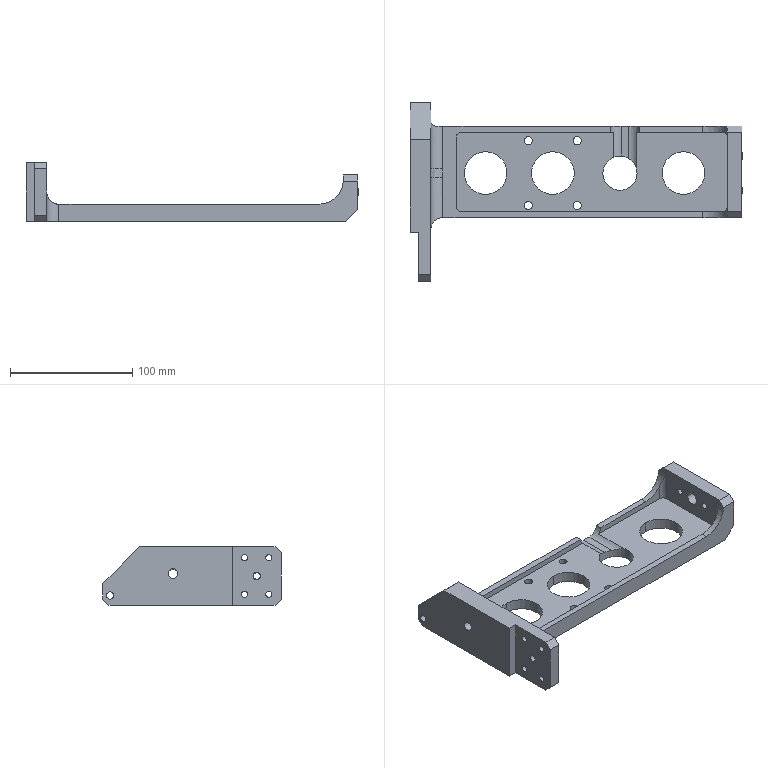Part | STEP file | J454-EBZ05-21-03-Part-1-4 | 1 solid | 92 faces | box 272 x 146 x 48 mm | volume 274570 mm3 | cylinder 58 | plane 33 | spline 1 | commonest cylinder face diameters 5 x12 6.6 x8 11 x8 8 x7 35 x6 6 x4